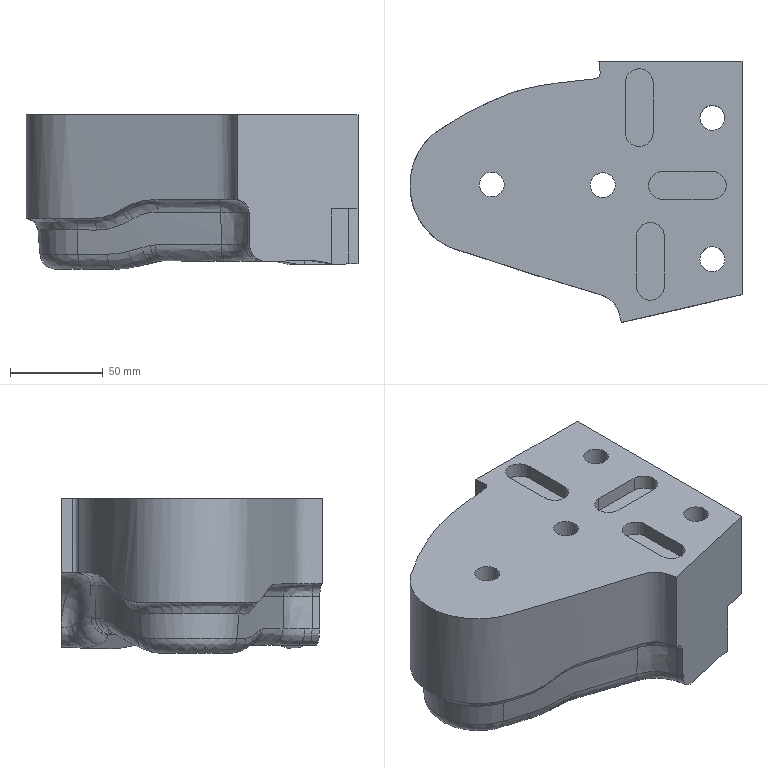Part | NX | features 8 2 | 1 solid | 122 faces | box 179.454 x 141.066 x 83.733 mm | volume 1222047 mm3 | spline 64 | plane 33 | cylinder 23 | cone 2 | commonest cylinder face diameters 15 x6 13.5 x4 20 x4 8.5 x3 14 x2 6 x1